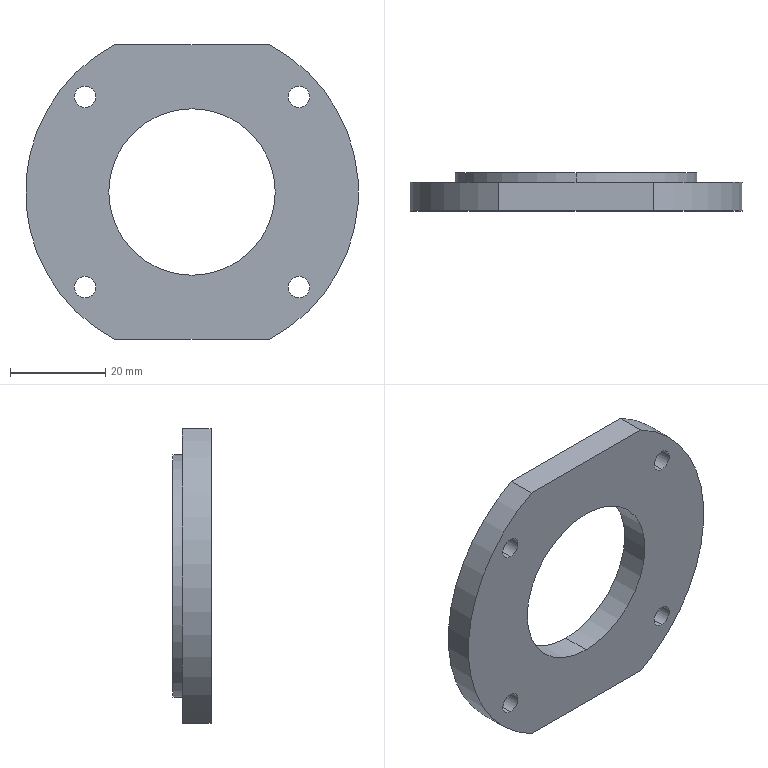Part | SolidWorks | features HoleWzd 1, ICE 1, Revolution 1 | 1 solid | 24 faces | box 70 x 8 x 62 mm | volume 17164 mm3 | cylinder 16 | plane 6 | cone 2 | commonest cylinder face diameters 4.5 x8 35 x2 43 x2 51 x2 70 x2
STEP:
#1=CARTESIAN_POINT('',(22.5,6.,-17.75));
#2=VERTEX_POINT('',#1);
#3=CARTESIAN_POINT('',(22.5,6.,-22.25));
#4=VERTEX_POINT('',#3);
#5=CARTESIAN_POINT('',(22.5,6.,-20.));
#6=DIRECTION('',(0.,-1.,0.));
#7=DIRECTION('',(0.,0.,-1.));
#8=AXIS2_PLACEMENT_3D('',#5,#6,#7);
#9=CIRCLE('',#8,2.25);
#10=EDGE_CURVE('',#2,#4,#9,.T.);
#11=ORIENTED_EDGE('',*,*,#10,.F.);
#12=CARTESIAN_POINT('',(22.5,0.,-17.75));
#13=VERTEX_POINT('',#12);
#14=CARTESIAN_POINT('',(22.5,0.,-17.75));
#15=DIRECTION('',(0.,-1.,0.));
#16=VECTOR('',#15,1000.);
#17=LINE('',#14,#16);
#18=EDGE_CURVE('',#2,#13,#17,.T.);
#19=ORIENTED_EDGE('',*,*,#18,.T.);
#20=CARTESIAN_POINT('',(22.5,0.,-22.25));
#21=VERTEX_POINT('',#20);
#22=CARTESIAN_POINT('',(22.5,0.,-20.));
#23=DIRECTION('',(0.,-1.,0.));
#24=DIRECTION('',(0.,0.,-1.));
#25=AXIS2_PLACEMENT_3D('',#22,#23,#24);
#26=CIRCLE('',#25,2.25);
#27=EDGE_CURVE('',#13,#21,#26,.T.);
#28=ORIENTED_EDGE('',*,*,#27,.T.);
#29=CARTESIAN_POINT('',(22.5,0.,-22.25));
#30=DIRECTION('',(0.,-1.,0.));
#31=VECTOR('',#30,1000.);
#32=LINE('',#29,#31);
#33=EDGE_CURVE('',#4,#21,#32,.T.);
#34=ORIENTED_EDGE('',*,*,#33,.F.);
#35=EDGE_LOOP('',(#11,#19,#28,#34));
#36=FACE_OUTER_BOUND('',#35,.T.);
#37=CARTESIAN_POINT('',(22.5,0.,-20.));
#38=DIRECTION('',(0.,-1.,0.));
#39=DIRECTION('',(0.,0.,-1.));
#40=AXIS2_PLACEMENT_3D('',#37,#38,#39);
#41=CYLINDRICAL_SURFACE('',#40,2.25);
#42=ADVANCED_FACE('',(#36),#41,.F.);
#43=CARTESIAN_POINT('',(22.5,6.,22.25));
#44=VERTEX_POINT('',#43);
#45=CARTESIAN_POINT('',(22.5,6.,17.75));
#46=VERTEX_POINT('',#45);
#47=CARTESIAN_POINT('',(22.5,6.,20.));
#48=DIRECTION('',(0.,-1.,0.));
#49=DIRECTION('',(0.,0.,-1.));
#50=AXIS2_PLACEMENT_3D('',#47,#48,#49);
#51=CIRCLE('',#50,2.25);
#52=EDGE_CURVE('',#44,#46,#51,.T.);
#53=ORIENTED_EDGE('',*,*,#52,.F.);
#54=CARTESIAN_POINT('',(22.5,0.,22.25));
#55=VERTEX_POINT('',#54);
#56=CARTESIAN_POINT('',(22.5,0.,22.25));
#57=DIRECTION('',(0.,-1.,0.));
#58=VECTOR('',#57,1000.);
#59=LINE('',#56,#58);
#60=EDGE_CURVE('',#44,#55,#59,.T.);
#61=ORIENTED_EDGE('',*,*,#60,.T.);
#62=CARTESIAN_POINT('',(22.5,0.,17.75));
#63=VERTEX_POINT('',#62);
#64=CARTESIAN_POINT('',(22.5,0.,20.));
#65=DIRECTION('',(0.,-1.,0.));
#66=DIRECTION('',(0.,0.,-1.));
#67=AXIS2_PLACEMENT_3D('',#64,#65,#66);
#68=CIRCLE('',#67,2.25);
#69=EDGE_CURVE('',#55,#63,#68,.T.);
#70=ORIENTED_EDGE('',*,*,#69,.T.);
#71=CARTESIAN_POINT('',(22.5,0.,17.75));
#72=DIRECTION('',(0.,-1.,0.));
#73=VECTOR('',#72,1000.);
#74=LINE('',#71,#73);
#75=EDGE_CURVE('',#46,#63,#74,.T.);
#76=ORIENTED_EDGE('',*,*,#75,.F.);
#77=EDGE_LOOP('',(#53,#61,#70,#76));
#78=FACE_OUTER_BOUND('',#77,.T.);
#79=CARTESIAN_POINT('',(22.5,0.,20.));
#80=DIRECTION('',(0.,-1.,0.));
#81=DIRECTION('',(0.,0.,-1.));
#82=AXIS2_PLACEMENT_3D('',#79,#80,#81);
#83=CYLINDRICAL_SURFACE('',#82,2.25);
#84=ADVANCED_FACE('',(#78),#83,.F.);
#85=CARTESIAN_POINT('',(-22.5,6.,-17.75));
#86=VERTEX_POINT('',#85);
#87=CARTESIAN_POINT('',(-22.5,6.,-22.25));
#88=VERTEX_POINT('',#87);
#89=CARTESIAN_POINT('',(-22.5,6.,-20.));
#90=DIRECTION('',(0.,-1.,0.));
#91=DIRECTION('',(0.,0.,-1.));
#92=AXIS2_PLACEMENT_3D('',#89,#90,#91);
#93=CIRCLE('',#92,2.25);
#94=EDGE_CURVE('',#86,#88,#93,.T.);
#95=ORIENTED_EDGE('',*,*,#94,.F.);
#96=CARTESIAN_POINT('',(-22.5,0.,-17.75));
#97=VERTEX_POINT('',#96);
#98=CARTESIAN_POINT('',(-22.5,0.,-17.75));
#99=DIRECTION('',(0.,-1.,0.));
#100=VECTOR('',#99,1000.);
#101=LINE('',#98,#100);
#102=EDGE_CURVE('',#86,#97,#101,.T.);
#103=ORIENTED_EDGE('',*,*,#102,.T.);
#104=CARTESIAN_POINT('',(-22.5,0.,-22.25));
#105=VERTEX_POINT('',#104);
#106=CARTESIAN_POINT('',(-22.5,0.,-20.));
#107=DIRECTION('',(0.,-1.,0.));
#108=DIRECTION('',(0.,0.,-1.));
#109=AXIS2_PLACEMENT_3D('',#106,#107,#108);
#110=CIRCLE('',#109,2.25);
#111=EDGE_CURVE('',#97,#105,#110,.T.);
#112=ORIENTED_EDGE('',*,*,#111,.T.);
#113=CARTESIAN_POINT('',(-22.5,0.,-22.25));
#114=DIRECTION('',(0.,-1.,0.));
#115=VECTOR('',#114,1000.);
#116=LINE('',#113,#115);
#117=EDGE_CURVE('',#88,#105,#116,.T.);
#118=ORIENTED_EDGE('',*,*,#117,.F.);
#119=EDGE_LOOP('',(#95,#103,#112,#118));
#120=FACE_OUTER_BOUND('',#119,.T.);
#121=CARTESIAN_POINT('',(-22.5,0.,-20.));
#122=DIRECTION('',(0.,-1.,0.));
#123=DIRECTION('',(0.,0.,-1.));
#124=AXIS2_PLACEMENT_3D('',#121,#122,#123);
#125=CYLINDRICAL_SURFACE('',#124,2.25);
#126=ADVANCED_FACE('',(#120),#125,.F.);
#127=CARTESIAN_POINT('',(-22.5,6.,22.25));
#128=VERTEX_POINT('',#127);
#129=CARTESIAN_POINT('',(-22.5,6.,17.75));
#130=VERTEX_POINT('',#129);
#131=CARTESIAN_POINT('',(-22.5,6.,20.));
#132=DIRECTION('',(0.,-1.,0.));
#133=DIRECTION('',(0.,0.,-1.));
#134=AXIS2_PLACEMENT_3D('',#131,#132,#133);
#135=CIRCLE('',#134,2.25);
#136=EDGE_CURVE('',#128,#130,#135,.T.);
#137=ORIENTED_EDGE('',*,*,#136,.F.);
#138=CARTESIAN_POINT('',(-22.5,0.,22.25));
#139=VERTEX_POINT('',#138);
#140=CARTESIAN_POINT('',(-22.5,0.,22.25));
#141=DIRECTION('',(0.,-1.,0.));
#142=VECTOR('',#141,1000.);
#143=LINE('',#140,#142);
#144=EDGE_CURVE('',#128,#139,#143,.T.);
#145=ORIENTED_EDGE('',*,*,#144,.T.);
#146=CARTESIAN_POINT('',(-22.5,0.,17.75));
#147=VERTEX_POINT('',#146);
#148=CARTESIAN_POINT('',(-22.5,0.,20.));
#149=DIRECTION('',(0.,-1.,0.));
#150=DIRECTION('',(0.,0.,-1.));
#151=AXIS2_PLACEMENT_3D('',#148,#149,#150);
#152=CIRCLE('',#151,2.25);
#153=EDGE_CURVE('',#139,#147,#152,.T.);
#154=ORIENTED_EDGE('',*,*,#153,.T.);
#155=CARTESIAN_POINT('',(-22.5,0.,17.75));
#156=DIRECTION('',(0.,-1.,0.));
#157=VECTOR('',#156,1000.);
#158=LINE('',#155,#157);
#159=EDGE_CURVE('',#130,#147,#158,.T.);
#160=ORIENTED_EDGE('',*,*,#159,.F.);
#161=EDGE_LOOP('',(#137,#145,#154,#160));
#162=FACE_OUTER_BOUND('',#161,.T.);
#163=CARTESIAN_POINT('',(-22.5,0.,20.));
#164=DIRECTION('',(0.,-1.,0.));
#165=DIRECTION('',(0.,0.,-1.));
#166=AXIS2_PLACEMENT_3D('',#163,#164,#165);
#167=CYLINDRICAL_SURFACE('',#166,2.25);
#168=ADVANCED_FACE('',(#162),#167,.F.);
#169=CARTESIAN_POINT('',(0.,0.,-17.5));
#170=VERTEX_POINT('',#169);
#171=CARTESIAN_POINT('',(0.,0.,17.5));
#172=VERTEX_POINT('',#171);
#173=CARTESIAN_POINT('',(0.,0.,0.));
#174=DIRECTION('',(0.,1.,0.));
#175=DIRECTION('',(0.,0.,1.));
#176=AXIS2_PLACEMENT_3D('',#173,#174,#175);
#177=CIRCLE('',#176,17.5);
#178=EDGE_CURVE('',#170,#172,#177,.T.);
#179=ORIENTED_EDGE('',*,*,#178,.F.);
#180=CARTESIAN_POINT('',(0.,6.,-17.5));
#181=VERTEX_POINT('',#180);
#182=CARTESIAN_POINT('',(0.,112.431,-17.5));
#183=DIRECTION('',(0.,1.,0.));
#184=VECTOR('',#183,1000.);
#185=LINE('',#182,#184);
#186=EDGE_CURVE('',#170,#181,#185,.T.);
#187=ORIENTED_EDGE('',*,*,#186,.T.);
#188=CARTESIAN_POINT('',(0.,6.,17.5));
#189=VERTEX_POINT('',#188);
#190=CARTESIAN_POINT('',(0.,6.,0.));
#191=DIRECTION('',(0.,1.,0.));
#192=DIRECTION('',(0.,0.,1.));
#193=AXIS2_PLACEMENT_3D('',#190,#191,#192);
#194=CIRCLE('',#193,17.5);
#195=EDGE_CURVE('',#181,#189,#194,.T.);
#196=ORIENTED_EDGE('',*,*,#195,.T.);
#197=CARTESIAN_POINT('',(0.,112.431,17.5));
#198=DIRECTION('',(0.,1.,0.));
#199=VECTOR('',#198,1000.);
#200=LINE('',#197,#199);
#201=EDGE_CURVE('',#172,#189,#200,.T.);
#202=ORIENTED_EDGE('',*,*,#201,.F.);
#203=EDGE_LOOP('',(#179,#187,#196,#202));
#204=FACE_OUTER_BOUND('',#203,.T.);
#205=CARTESIAN_POINT('',(0.,112.431,0.));
#206=DIRECTION('',(0.,1.,0.));
#207=DIRECTION('',(0.,0.,1.));
#208=AXIS2_PLACEMENT_3D('',#205,#206,#207);
#209=CYLINDRICAL_SURFACE('',#208,17.5);
#210=ADVANCED_FACE('',(#204),#209,.F.);
#211=CARTESIAN_POINT('',(0.,6.,25.5));
#212=VERTEX_POINT('',#211);
#213=CARTESIAN_POINT('',(0.,6.,-25.5));
#214=VERTEX_POINT('',#213);
#215=CARTESIAN_POINT('',(0.,6.,0.));
#216=DIRECTION('',(0.,1.,0.));
#217=DIRECTION('',(0.,0.,1.));
#218=AXIS2_PLACEMENT_3D('',#215,#216,#217);
#219=CIRCLE('',#218,25.5);
#220=EDGE_CURVE('',#212,#214,#219,.T.);
#221=ORIENTED_EDGE('',*,*,#220,.T.);
#222=CARTESIAN_POINT('',(0.,8.,-25.5));
#223=VERTEX_POINT('',#222);
#224=CARTESIAN_POINT('',(0.,112.431,-25.5));
#225=DIRECTION('',(0.,1.,0.));
#226=VECTOR('',#225,1000.);
#227=LINE('',#224,#226);
#228=EDGE_CURVE('',#214,#223,#227,.T.);
#229=ORIENTED_EDGE('',*,*,#228,.T.);
#230=CARTESIAN_POINT('',(0.,8.,25.5));
#231=VERTEX_POINT('',#230);
#232=CARTESIAN_POINT('',(0.,8.,0.));
#233=DIRECTION('',(0.,1.,0.));
#234=DIRECTION('',(0.,0.,1.));
#235=AXIS2_PLACEMENT_3D('',#232,#233,#234);
#236=CIRCLE('',#235,25.5);
#237=EDGE_CURVE('',#231,#223,#236,.T.);
#238=ORIENTED_EDGE('',*,*,#237,.F.);
#239=CARTESIAN_POINT('',(0.,112.431,25.5));
#240=DIRECTION('',(0.,1.,0.));
#241=VECTOR('',#240,1000.);
#242=LINE('',#239,#241);
#243=EDGE_CURVE('',#212,#231,#242,.T.);
#244=ORIENTED_EDGE('',*,*,#243,.F.);
#245=EDGE_LOOP('',(#221,#229,#238,#244));
#246=FACE_OUTER_BOUND('',#245,.T.);
#247=CARTESIAN_POINT('',(0.,112.431,0.));
#248=DIRECTION('',(0.,1.,0.));
#249=DIRECTION('',(0.,0.,1.));
#250=AXIS2_PLACEMENT_3D('',#247,#248,#249);
#251=CYLINDRICAL_SURFACE('',#250,25.5);
#252=ADVANCED_FACE('',(#246),#251,.T.);
#253=CARTESIAN_POINT('',(0.,7.,-21.5));
#254=VERTEX_POINT('',#253);
#255=CARTESIAN_POINT('',(0.,7.,21.5));
#256=VERTEX_POINT('',#255);
#257=CARTESIAN_POINT('',(0.,7.,0.));
#258=DIRECTION('',(0.,1.,0.));
#259=DIRECTION('',(0.,0.,1.));
#260=AXIS2_PLACEMENT_3D('',#257,#258,#259);
#261=CIRCLE('',#260,21.5);
#262=EDGE_CURVE('',#254,#256,#261,.T.);
#263=ORIENTED_EDGE('',*,*,#262,.F.);
#264=CARTESIAN_POINT('',(0.,8.,-21.5));
#265=VERTEX_POINT('',#264);
#266=CARTESIAN_POINT('',(0.,112.431,-21.5));
#267=DIRECTION('',(0.,1.,0.));
#268=VECTOR('',#267,1000.);
#269=LINE('',#266,#268);
#270=EDGE_CURVE('',#254,#265,#269,.T.);
#271=ORIENTED_EDGE('',*,*,#270,.T.);
#272=CARTESIAN_POINT('',(0.,8.,21.5));
#273=VERTEX_POINT('',#272);
#274=CARTESIAN_POINT('',(0.,8.,0.));
#275=DIRECTION('',(0.,1.,0.));
#276=DIRECTION('',(0.,0.,1.));
#277=AXIS2_PLACEMENT_3D('',#274,#275,#276);
#278=CIRCLE('',#277,21.5);
#279=EDGE_CURVE('',#265,#273,#278,.T.);
#280=ORIENTED_EDGE('',*,*,#279,.T.);
#281=CARTESIAN_POINT('',(0.,112.431,21.5));
#282=DIRECTION('',(0.,1.,0.));
#283=VECTOR('',#282,1000.);
#284=LINE('',#281,#283);
#285=EDGE_CURVE('',#256,#273,#284,.T.);
#286=ORIENTED_EDGE('',*,*,#285,.F.);
#287=EDGE_LOOP('',(#263,#271,#280,#286));
#288=FACE_OUTER_BOUND('',#287,.T.);
#289=CARTESIAN_POINT('',(0.,112.431,0.));
#290=DIRECTION('',(0.,1.,0.));
#291=DIRECTION('',(0.,0.,1.));
#292=AXIS2_PLACEMENT_3D('',#289,#290,#291);
#293=CYLINDRICAL_SURFACE('',#292,21.5);
#294=ADVANCED_FACE('',(#288),#293,.F.);
#295=CARTESIAN_POINT('',(0.,6.,-20.));
#296=VERTEX_POINT('',#295);
#297=CARTESIAN_POINT('',(0.,6.,20.));
#298=VERTEX_POINT('',#297);
#299=CARTESIAN_POINT('',(0.,6.,0.));
#300=DIRECTION('',(0.,1.,0.));
#301=DIRECTION('',(0.,0.,1.));
#302=AXIS2_PLACEMENT_3D('',#299,#300,#301);
#303=CIRCLE('',#302,20.);
#304=EDGE_CURVE('',#296,#298,#303,.T.);
#305=ORIENTED_EDGE('',*,*,#304,.F.);
#306=CARTESIAN_POINT('',(0.,7.,-21.5));
#307=DIRECTION('',(0.,0.5547,-0.8321));
#308=VECTOR('',#307,1000.);
#309=LINE('',#306,#308);
#310=EDGE_CURVE('',#296,#254,#309,.T.);
#311=ORIENTED_EDGE('',*,*,#310,.T.);
#312=ORIENTED_EDGE('',*,*,#262,.T.);
#313=CARTESIAN_POINT('',(0.,7.,21.5));
#314=DIRECTION('',(0.,0.5547,0.8321));
#315=VECTOR('',#314,1000.);
#316=LINE('',#313,#315);
#317=EDGE_CURVE('',#298,#256,#316,.T.);
#318=ORIENTED_EDGE('',*,*,#317,.F.);
#319=EDGE_LOOP('',(#305,#311,#312,#318));
#320=FACE_OUTER_BOUND('',#319,.T.);
#321=CARTESIAN_POINT('',(0.,7.,0.));
#322=DIRECTION('',(0.,1.,0.));
#323=DIRECTION('',(0.,0.,1.));
#324=AXIS2_PLACEMENT_3D('',#321,#322,#323);
#325=CONICAL_SURFACE('',#324,21.5,0.9828);
#326=ADVANCED_FACE('',(#320),#325,.F.);
#327=CARTESIAN_POINT('',(0.,0.,0.));
#328=DIRECTION('',(0.,1.,0.));
#329=DIRECTION('',(0.,0.,1.));
#330=AXIS2_PLACEMENT_3D('',#327,#328,#329);
#331=CIRCLE('',#330,17.5);
#332=EDGE_CURVE('',#172,#170,#331,.T.);
#333=ORIENTED_EDGE('',*,*,#332,.T.);
#334=ORIENTED_EDGE('',*,*,#178,.T.);
#335=EDGE_LOOP('',(#333,#334));
#336=FACE_BOUND('',#335,.T.);
#337=CARTESIAN_POINT('',(-22.5,0.,20.));
#338=DIRECTION('',(0.,-1.,0.));
#339=DIRECTION('',(0.,0.,-1.));
#340=AXIS2_PLACEMENT_3D('',#337,#338,#339);
#341=CIRCLE('',#340,2.25);
#342=EDGE_CURVE('',#147,#139,#341,.T.);
#343=ORIENTED_EDGE('',*,*,#342,.F.);
#344=ORIENTED_EDGE('',*,*,#153,.F.);
#345=EDGE_LOOP('',(#343,#344));
#346=FACE_BOUND('',#345,.T.);
#347=CARTESIAN_POINT('',(-22.5,0.,-20.));
#348=DIRECTION('',(0.,-1.,0.));
#349=DIRECTION('',(0.,0.,-1.));
#350=AXIS2_PLACEMENT_3D('',#347,#348,#349);
#351=CIRCLE('',#350,2.25);
#352=EDGE_CURVE('',#105,#97,#351,.T.);
#353=ORIENTED_EDGE('',*,*,#352,.F.);
#354=ORIENTED_EDGE('',*,*,#111,.F.);
#355=EDGE_LOOP('',(#353,#354));
#356=FACE_BOUND('',#355,.T.);
#357=CARTESIAN_POINT('',(22.5,0.,20.));
#358=DIRECTION('',(0.,-1.,0.));
#359=DIRECTION('',(0.,0.,-1.));
#360=AXIS2_PLACEMENT_3D('',#357,#358,#359);
#361=CIRCLE('',#360,2.25);
#362=EDGE_CURVE('',#63,#55,#361,.T.);
#363=ORIENTED_EDGE('',*,*,#362,.F.);
#364=ORIENTED_EDGE('',*,*,#69,.F.);
#365=EDGE_LOOP('',(#363,#364));
#366=FACE_BOUND('',#365,.T.);
#367=CARTESIAN_POINT('',(22.5,0.,-20.));
#368=DIRECTION('',(0.,-1.,0.));
#369=DIRECTION('',(0.,0.,-1.));
#370=AXIS2_PLACEMENT_3D('',#367,#368,#369);
#371=CIRCLE('',#370,2.25);
#372=EDGE_CURVE('',#21,#13,#371,.T.);
#373=ORIENTED_EDGE('',*,*,#372,.F.);
#374=ORIENTED_EDGE('',*,*,#27,.F.);
#375=EDGE_LOOP('',(#373,#374));
#376=FACE_BOUND('',#375,.T.);
#377=CARTESIAN_POINT('',(16.248,0.,31.));
#378=VERTEX_POINT('',#377);
#379=CARTESIAN_POINT('',(-16.248,0.,31.));
#380=VERTEX_POINT('',#379);
#381=CARTESIAN_POINT('',(41.782,0.,31.));
#382=DIRECTION('',(-1.,0.,0.));
#383=VECTOR('',#382,1000.);
#384=LINE('',#381,#383);
#385=EDGE_CURVE('',#378,#380,#384,.T.);
#386=ORIENTED_EDGE('',*,*,#385,.T.);
#387=CARTESIAN_POINT('',(-16.248,0.,-31.));
#388=VERTEX_POINT('',#387);
#389=CARTESIAN_POINT('',(0.,0.,0.));
#390=DIRECTION('',(0.,1.,0.));
#391=DIRECTION('',(0.,0.,1.));
#392=AXIS2_PLACEMENT_3D('',#389,#390,#391);
#393=CIRCLE('',#392,35.);
#394=EDGE_CURVE('',#388,#380,#393,.T.);
#395=ORIENTED_EDGE('',*,*,#394,.F.);
#396=CARTESIAN_POINT('',(16.248,0.,-31.));
#397=VERTEX_POINT('',#396);
#398=CARTESIAN_POINT('',(41.782,0.,-31.));
#399=DIRECTION('',(1.,0.,0.));
#400=VECTOR('',#399,1000.);
#401=LINE('',#398,#400);
#402=EDGE_CURVE('',#388,#397,#401,.T.);
#403=ORIENTED_EDGE('',*,*,#402,.T.);
#404=CARTESIAN_POINT('',(0.,0.,0.));
#405=DIRECTION('',(0.,1.,0.));
#406=DIRECTION('',(0.,0.,1.));
#407=AXIS2_PLACEMENT_3D('',#404,#405,#406);
#408=CIRCLE('',#407,35.);
#409=EDGE_CURVE('',#378,#397,#408,.T.);
#410=ORIENTED_EDGE('',*,*,#409,.F.);
#411=EDGE_LOOP('',(#386,#395,#403,#410));
#412=FACE_OUTER_BOUND('',#411,.T.);
#413=CARTESIAN_POINT('',(17.5,0.,0.));
#414=DIRECTION('',(0.,1.,0.));
#415=DIRECTION('',(0.,0.,1.));
#416=AXIS2_PLACEMENT_3D('',#413,#414,#415);
#417=PLANE('',#416);
#418=ADVANCED_FACE('',(#336,#346,#356,#366,#376,#412),#417,.F.);
#419=CARTESIAN_POINT('',(22.5,6.,-20.));
#420=DIRECTION('',(0.,-1.,0.));
#421=DIRECTION('',(0.,0.,-1.));
#422=AXIS2_PLACEMENT_3D('',#419,#420,#421);
#423=CIRCLE('',#422,2.25);
#424=EDGE_CURVE('',#4,#2,#423,.T.);
#425=ORIENTED_EDGE('',*,*,#424,.T.);
#426=ORIENTED_EDGE('',*,*,#10,.T.);
#427=EDGE_LOOP('',(#425,#426));
#428=FACE_BOUND('',#427,.T.);
#429=CARTESIAN_POINT('',(22.5,6.,20.));
#430=DIRECTION('',(0.,-1.,0.));
#431=DIRECTION('',(0.,0.,-1.));
#432=AXIS2_PLACEMENT_3D('',#429,#430,#431);
#433=CIRCLE('',#432,2.25);
#434=EDGE_CURVE('',#46,#44,#433,.T.);
#435=ORIENTED_EDGE('',*,*,#434,.T.);
#436=ORIENTED_EDGE('',*,*,#52,.T.);
#437=EDGE_LOOP('',(#435,#436));
#438=FACE_BOUND('',#437,.T.);
#439=CARTESIAN_POINT('',(-22.5,6.,-20.));
#440=DIRECTION('',(0.,-1.,0.));
#441=DIRECTION('',(0.,0.,-1.));
#442=AXIS2_PLACEMENT_3D('',#439,#440,#441);
#443=CIRCLE('',#442,2.25);
#444=EDGE_CURVE('',#88,#86,#443,.T.);
#445=ORIENTED_EDGE('',*,*,#444,.T.);
#446=ORIENTED_EDGE('',*,*,#94,.T.);
#447=EDGE_LOOP('',(#445,#446));
#448=FACE_BOUND('',#447,.T.);
#449=CARTESIAN_POINT('',(-22.5,6.,20.));
#450=DIRECTION('',(0.,-1.,0.));
#451=DIRECTION('',(0.,0.,-1.));
#452=AXIS2_PLACEMENT_3D('',#449,#450,#451);
#453=CIRCLE('',#452,2.25);
#454=EDGE_CURVE('',#130,#128,#453,.T.);
#455=ORIENTED_EDGE('',*,*,#454,.T.);
#456=ORIENTED_EDGE('',*,*,#136,.T.);
#457=EDGE_LOOP('',(#455,#456));
#458=FACE_BOUND('',#457,.T.);
#459=ORIENTED_EDGE('',*,*,#220,.F.);
#460=CARTESIAN_POINT('',(0.,6.,0.));
#461=DIRECTION('',(0.,1.,0.));
#462=DIRECTION('',(0.,0.,1.));
#463=AXIS2_PLACEMENT_3D('',#460,#461,#462);
#464=CIRCLE('',#463,25.5);
#465=EDGE_CURVE('',#214,#212,#464,.T.);
#466=ORIENTED_EDGE('',*,*,#465,.F.);
#467=EDGE_LOOP('',(#459,#466));
#468=FACE_BOUND('',#467,.T.);
#469=CARTESIAN_POINT('',(16.248,6.,31.));
#470=VERTEX_POINT('',#469);
#471=CARTESIAN_POINT('',(-16.248,6.,31.));
#472=VERTEX_POINT('',#471);
#473=CARTESIAN_POINT('',(25.5,6.,31.));
#474=DIRECTION('',(-1.,0.,0.));
#475=VECTOR('',#474,1000.);
#476=LINE('',#473,#475);
#477=EDGE_CURVE('',#470,#472,#476,.T.);
#478=ORIENTED_EDGE('',*,*,#477,.F.);
#479=CARTESIAN_POINT('',(16.248,6.,-31.));
#480=VERTEX_POINT('',#479);
#481=CARTESIAN_POINT('',(0.,6.,0.));
#482=DIRECTION('',(0.,1.,0.));
#483=DIRECTION('',(0.,0.,1.));
#484=AXIS2_PLACEMENT_3D('',#481,#482,#483);
#485=CIRCLE('',#484,35.);
#486=EDGE_CURVE('',#470,#480,#485,.T.);
#487=ORIENTED_EDGE('',*,*,#486,.T.);
#488=CARTESIAN_POINT('',(-16.248,6.,-31.));
#489=VERTEX_POINT('',#488);
#490=CARTESIAN_POINT('',(25.5,6.,-31.));
#491=DIRECTION('',(1.,0.,0.));
#492=VECTOR('',#491,1000.);
#493=LINE('',#490,#492);
#494=EDGE_CURVE('',#489,#480,#493,.T.);
#495=ORIENTED_EDGE('',*,*,#494,.F.);
#496=CARTESIAN_POINT('',(0.,6.,0.));
#497=DIRECTION('',(0.,1.,0.));
#498=DIRECTION('',(0.,0.,1.));
#499=AXIS2_PLACEMENT_3D('',#496,#497,#498);
#500=CIRCLE('',#499,35.);
#501=EDGE_CURVE('',#489,#472,#500,.T.);
#502=ORIENTED_EDGE('',*,*,#501,.T.);
#503=EDGE_LOOP('',(#478,#487,#495,#502));
#504=FACE_OUTER_BOUND('',#503,.T.);
#505=CARTESIAN_POINT('',(25.5,6.,0.));
#506=DIRECTION('',(0.,-1.,0.));
#507=DIRECTION('',(0.,0.,-1.));
#508=AXIS2_PLACEMENT_3D('',#505,#506,#507);
#509=PLANE('',#508);
#510=ADVANCED_FACE('',(#428,#438,#448,#458,#468,#504),#509,.F.);
#511=CARTESIAN_POINT('',(16.248,112.431,31.));
#512=DIRECTION('',(0.,1.,0.));
#513=VECTOR('',#512,1000.);
#514=LINE('',#511,#513);
#515=EDGE_CURVE('',#378,#470,#514,.T.);
#516=ORIENTED_EDGE('',*,*,#515,.F.);
#517=ORIENTED_EDGE('',*,*,#409,.T.);
#518=CARTESIAN_POINT('',(16.248,112.431,-31.));
#519=DIRECTION('',(0.,-1.,0.));
#520=VECTOR('',#519,1000.);
#521=LINE('',#518,#520);
#522=EDGE_CURVE('',#480,#397,#521,.T.);
#523=ORIENTED_EDGE('',*,*,#522,.F.);
#524=ORIENTED_EDGE('',*,*,#486,.F.);
#525=EDGE_LOOP('',(#516,#517,#523,#524));
#526=FACE_OUTER_BOUND('',#525,.T.);
#527=CARTESIAN_POINT('',(0.,112.431,0.));
#528=DIRECTION('',(0.,1.,0.));
#529=DIRECTION('',(0.,0.,1.));
#530=AXIS2_PLACEMENT_3D('',#527,#528,#529);
#531=CYLINDRICAL_SURFACE('',#530,35.);
#532=ADVANCED_FACE('',(#526),#531,.T.);
#533=CARTESIAN_POINT('',(-16.248,112.431,31.));
#534=DIRECTION('',(0.,-1.,0.));
#535=VECTOR('',#534,1000.);
#536=LINE('',#533,#535);
#537=EDGE_CURVE('',#472,#380,#536,.T.);
#538=ORIENTED_EDGE('',*,*,#537,.F.);
#539=ORIENTED_EDGE('',*,*,#501,.F.);
#540=CARTESIAN_POINT('',(-16.248,112.431,-31.));
#541=DIRECTION('',(0.,1.,0.));
#542=VECTOR('',#541,1000.);
#543=LINE('',#540,#542);
#544=EDGE_CURVE('',#388,#489,#543,.T.);
#545=ORIENTED_EDGE('',*,*,#544,.F.);
#546=ORIENTED_EDGE('',*,*,#394,.T.);
#547=EDGE_LOOP('',(#538,#539,#545,#546));
#548=FACE_OUTER_BOUND('',#547,.T.);
#549=CARTESIAN_POINT('',(0.,112.431,0.));
#550=DIRECTION('',(0.,1.,0.));
#551=DIRECTION('',(0.,0.,1.));
#552=AXIS2_PLACEMENT_3D('',#549,#550,#551);
#553=CYLINDRICAL_SURFACE('',#552,35.);
#554=ADVANCED_FACE('',(#548),#553,.T.);
#555=CARTESIAN_POINT('',(0.,6.,0.));
#556=DIRECTION('',(0.,1.,0.));
#557=DIRECTION('',(0.,0.,1.));
#558=AXIS2_PLACEMENT_3D('',#555,#556,#557);
#559=CIRCLE('',#558,17.5);
#560=EDGE_CURVE('',#189,#181,#559,.T.);
#561=ORIENTED_EDGE('',*,*,#560,.F.);
#562=ORIENTED_EDGE('',*,*,#195,.F.);
#563=EDGE_LOOP('',(#561,#562));
#564=FACE_BOUND('',#563,.T.);
#565=CARTESIAN_POINT('',(0.,6.,0.));
#566=DIRECTION('',(0.,1.,0.));
#567=DIRECTION('',(0.,0.,1.));
#568=AXIS2_PLACEMENT_3D('',#565,#566,#567);
#569=CIRCLE('',#568,20.);
#570=EDGE_CURVE('',#298,#296,#569,.T.);
#571=ORIENTED_EDGE('',*,*,#570,.T.);
#572=ORIENTED_EDGE('',*,*,#304,.T.);
#573=EDGE_LOOP('',(#571,#572));
#574=FACE_OUTER_BOUND('',#573,.T.);
#575=CARTESIAN_POINT('',(20.,6.,0.));
#576=DIRECTION('',(0.,-1.,0.));
#577=DIRECTION('',(0.,0.,-1.));
#578=AXIS2_PLACEMENT_3D('',#575,#576,#577);
#579=PLANE('',#578);
#580=ADVANCED_FACE('',(#564,#574),#579,.F.);
#581=ORIENTED_EDGE('',*,*,#310,.F.);
#582=ORIENTED_EDGE('',*,*,#570,.F.);
#583=ORIENTED_EDGE('',*,*,#317,.T.);
#584=CARTESIAN_POINT('',(0.,7.,0.));
#585=DIRECTION('',(0.,1.,0.));
#586=DIRECTION('',(0.,0.,1.));
#587=AXIS2_PLACEMENT_3D('',#584,#585,#586);
#588=CIRCLE('',#587,21.5);
#589=EDGE_CURVE('',#256,#254,#588,.T.);
#590=ORIENTED_EDGE('',*,*,#589,.T.);
#591=EDGE_LOOP('',(#581,#582,#583,#590));
#592=FACE_OUTER_BOUND('',#591,.T.);
#593=CARTESIAN_POINT('',(0.,7.,0.));
#594=DIRECTION('',(0.,1.,0.));
#595=DIRECTION('',(0.,0.,1.));
#596=AXIS2_PLACEMENT_3D('',#593,#594,#595);
#597=CONICAL_SURFACE('',#596,21.5,0.9828);
#598=ADVANCED_FACE('',(#592),#597,.F.);
#599=ORIENTED_EDGE('',*,*,#270,.F.);
#600=ORIENTED_EDGE('',*,*,#589,.F.);
#601=ORIENTED_EDGE('',*,*,#285,.T.);
#602=CARTESIAN_POINT('',(0.,8.,0.));
#603=DIRECTION('',(0.,1.,0.));
#604=DIRECTION('',(0.,0.,1.));
#605=AXIS2_PLACEMENT_3D('',#602,#603,#604);
#606=CIRCLE('',#605,21.5);
#607=EDGE_CURVE('',#273,#265,#606,.T.);
#608=ORIENTED_EDGE('',*,*,#607,.T.);
#609=EDGE_LOOP('',(#599,#600,#601,#608));
#610=FACE_OUTER_BOUND('',#609,.T.);
#611=CARTESIAN_POINT('',(0.,112.431,0.));
#612=DIRECTION('',(0.,1.,0.));
#613=DIRECTION('',(0.,0.,1.));
#614=AXIS2_PLACEMENT_3D('',#611,#612,#613);
#615=CYLINDRICAL_SURFACE('',#614,21.5);
#616=ADVANCED_FACE('',(#610),#615,.F.);
#617=ORIENTED_EDGE('',*,*,#607,.F.);
#618=ORIENTED_EDGE('',*,*,#279,.F.);
#619=EDGE_LOOP('',(#617,#618));
#620=FACE_BOUND('',#619,.T.);
#621=ORIENTED_EDGE('',*,*,#237,.T.);
#622=CARTESIAN_POINT('',(0.,8.,0.));
#623=DIRECTION('',(0.,1.,0.));
#624=DIRECTION('',(0.,0.,1.));
#625=AXIS2_PLACEMENT_3D('',#622,#623,#624);
#626=CIRCLE('',#625,25.5);
#627=EDGE_CURVE('',#223,#231,#626,.T.);
#628=ORIENTED_EDGE('',*,*,#627,.T.);
#629=EDGE_LOOP('',(#621,#628));
#630=FACE_OUTER_BOUND('',#629,.T.);
#631=CARTESIAN_POINT('',(25.5,8.,0.));
#632=DIRECTION('',(0.,-1.,0.));
#633=DIRECTION('',(0.,0.,-1.));
#634=AXIS2_PLACEMENT_3D('',#631,#632,#633);
#635=PLANE('',#634);
#636=ADVANCED_FACE('',(#620,#630),#635,.F.);
#637=ORIENTED_EDGE('',*,*,#228,.F.);
#638=ORIENTED_EDGE('',*,*,#465,.T.);
#639=ORIENTED_EDGE('',*,*,#243,.T.);
#640=ORIENTED_EDGE('',*,*,#627,.F.);
#641=EDGE_LOOP('',(#637,#638,#639,#640));
#642=FACE_OUTER_BOUND('',#641,.T.);
#643=CARTESIAN_POINT('',(0.,112.431,0.));
#644=DIRECTION('',(0.,1.,0.));
#645=DIRECTION('',(0.,0.,1.));
#646=AXIS2_PLACEMENT_3D('',#643,#644,#645);
#647=CYLINDRICAL_SURFACE('',#646,25.5);
#648=ADVANCED_FACE('',(#642),#647,.T.);
#649=ORIENTED_EDGE('',*,*,#186,.F.);
#650=ORIENTED_EDGE('',*,*,#332,.F.);
#651=ORIENTED_EDGE('',*,*,#201,.T.);
#652=ORIENTED_EDGE('',*,*,#560,.T.);
#653=EDGE_LOOP('',(#649,#650,#651,#652));
#654=FACE_OUTER_BOUND('',#653,.T.);
#655=CARTESIAN_POINT('',(0.,112.431,0.));
#656=DIRECTION('',(0.,1.,0.));
#657=DIRECTION('',(0.,0.,1.));
#658=AXIS2_PLACEMENT_3D('',#655,#656,#657);
#659=CYLINDRICAL_SURFACE('',#658,17.5);
#660=ADVANCED_FACE('',(#654),#659,.F.);
#661=ORIENTED_EDGE('',*,*,#144,.F.);
#662=ORIENTED_EDGE('',*,*,#454,.F.);
#663=ORIENTED_EDGE('',*,*,#159,.T.);
#664=ORIENTED_EDGE('',*,*,#342,.T.);
#665=EDGE_LOOP('',(#661,#662,#663,#664));
#666=FACE_OUTER_BOUND('',#665,.T.);
#667=CARTESIAN_POINT('',(-22.5,0.,20.));
#668=DIRECTION('',(0.,-1.,0.));
#669=DIRECTION('',(0.,0.,-1.));
#670=AXIS2_PLACEMENT_3D('',#667,#668,#669);
#671=CYLINDRICAL_SURFACE('',#670,2.25);
#672=ADVANCED_FACE('',(#666),#671,.F.);
#673=ORIENTED_EDGE('',*,*,#102,.F.);
#674=ORIENTED_EDGE('',*,*,#444,.F.);
#675=ORIENTED_EDGE('',*,*,#117,.T.);
#676=ORIENTED_EDGE('',*,*,#352,.T.);
#677=EDGE_LOOP('',(#673,#674,#675,#676));
#678=FACE_OUTER_BOUND('',#677,.T.);
#679=CARTESIAN_POINT('',(-22.5,0.,-20.));
#680=DIRECTION('',(0.,-1.,0.));
#681=DIRECTION('',(0.,0.,-1.));
#682=AXIS2_PLACEMENT_3D('',#679,#680,#681);
#683=CYLINDRICAL_SURFACE('',#682,2.25);
#684=ADVANCED_FACE('',(#678),#683,.F.);
#685=ORIENTED_EDGE('',*,*,#60,.F.);
#686=ORIENTED_EDGE('',*,*,#434,.F.);
#687=ORIENTED_EDGE('',*,*,#75,.T.);
#688=ORIENTED_EDGE('',*,*,#362,.T.);
#689=EDGE_LOOP('',(#685,#686,#687,#688));
#690=FACE_OUTER_BOUND('',#689,.T.);
#691=CARTESIAN_POINT('',(22.5,0.,20.));
#692=DIRECTION('',(0.,-1.,0.));
#693=DIRECTION('',(0.,0.,-1.));
#694=AXIS2_PLACEMENT_3D('',#691,#692,#693);
#695=CYLINDRICAL_SURFACE('',#694,2.25);
#696=ADVANCED_FACE('',(#690),#695,.F.);
#697=ORIENTED_EDGE('',*,*,#18,.F.);
#698=ORIENTED_EDGE('',*,*,#424,.F.);
#699=ORIENTED_EDGE('',*,*,#33,.T.);
#700=ORIENTED_EDGE('',*,*,#372,.T.);
#701=EDGE_LOOP('',(#697,#698,#699,#700));
#702=FACE_OUTER_BOUND('',#701,.T.);
#703=CARTESIAN_POINT('',(22.5,0.,-20.));
#704=DIRECTION('',(0.,-1.,0.));
#705=DIRECTION('',(0.,0.,-1.));
#706=AXIS2_PLACEMENT_3D('',#703,#704,#705);
#707=CYLINDRICAL_SURFACE('',#706,2.25);
#708=ADVANCED_FACE('',(#702),#707,.F.);
#709=ORIENTED_EDGE('',*,*,#544,.T.);
#710=ORIENTED_EDGE('',*,*,#494,.T.);
#711=ORIENTED_EDGE('',*,*,#522,.T.);
#712=ORIENTED_EDGE('',*,*,#402,.F.);
#713=EDGE_LOOP('',(#709,#710,#711,#712));
#714=FACE_OUTER_BOUND('',#713,.T.);
#715=CARTESIAN_POINT('',(41.782,8.,-31.));
#716=DIRECTION('',(0.,0.,-1.));
#717=DIRECTION('',(-1.,0.,0.));
#718=AXIS2_PLACEMENT_3D('',#715,#716,#717);
#719=PLANE('',#718);
#720=ADVANCED_FACE('',(#714),#719,.T.);
#721=ORIENTED_EDGE('',*,*,#515,.T.);
#722=ORIENTED_EDGE('',*,*,#477,.T.);
#723=ORIENTED_EDGE('',*,*,#537,.T.);
#724=ORIENTED_EDGE('',*,*,#385,.F.);
#725=EDGE_LOOP('',(#721,#722,#723,#724));
#726=FACE_OUTER_BOUND('',#725,.T.);
#727=CARTESIAN_POINT('',(41.782,8.,31.));
#728=DIRECTION('',(0.,0.,1.));
#729=DIRECTION('',(1.,0.,0.));
#730=AXIS2_PLACEMENT_3D('',#727,#728,#729);
#731=PLANE('',#730);
#732=ADVANCED_FACE('',(#726),#731,.T.);
#733=CLOSED_SHELL('',(#42,#84,#126,#168,#210,#252,#294,#326,#418,#510,#532,#554,#580,#598,#616,#636,#648,#660,#672,#684,#696,#708,#720,#732));
#734=MANIFOLD_SOLID_BREP('',#733);
#735=CARTESIAN_POINT('',(0.,0.,0.));
#736=DIRECTION('',(0.,0.,1.));
#737=DIRECTION('',(1.,0.,0.));
#738=AXIS2_PLACEMENT_3D('',#735,#736,#737);
#739=(LENGTH_UNIT()NAMED_UNIT(*)SI_UNIT(.MILLI.,.METRE.));
#740=UNCERTAINTY_MEASURE_WITH_UNIT(LENGTH_MEASURE(0.00001),#739,'','');
#741=(NAMED_UNIT(*)PLANE_ANGLE_UNIT()SI_UNIT($,.RADIAN.));
#742=(NAMED_UNIT(*)SI_UNIT($,.STERADIAN.)SOLID_ANGLE_UNIT());
#743=(GEOMETRIC_REPRESENTATION_CONTEXT(3)GLOBAL_UNCERTAINTY_ASSIGNED_CONTEXT((#740))GLOBAL_UNIT_ASSIGNED_CONTEXT((#739,#741,#742))REPRESENTATION_CONTEXT('',''));
#744=ADVANCED_BREP_SHAPE_REPRESENTATION('',(#734,#738),#743);